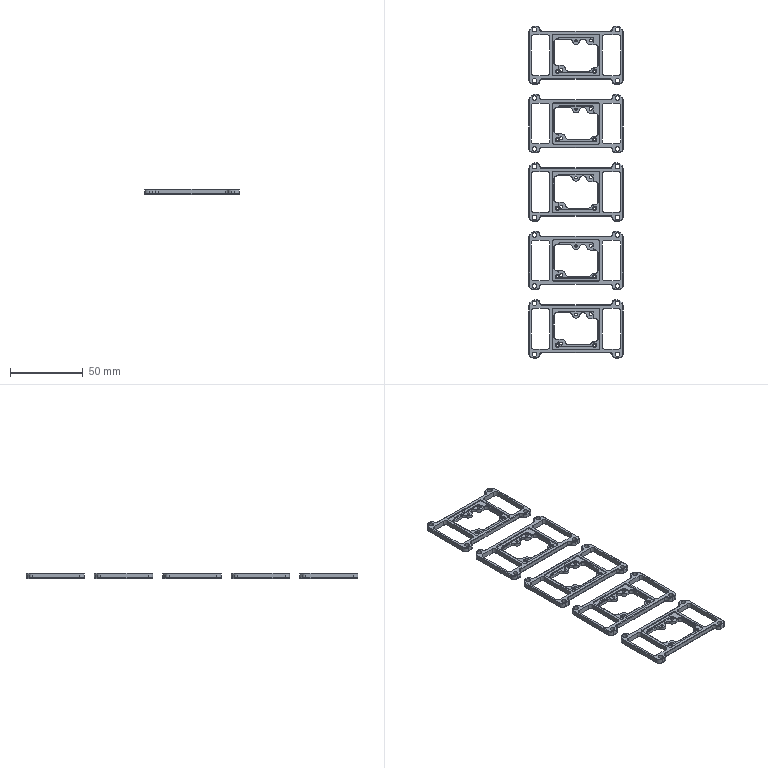Part | 5 solids | 970 faces | box 65 x 228 x 3.5 mm | volume 14203 mm3 | cylinder 395 | plane 335 | cone 170 | torus 70 | commonest cylinder face diameters 4 x125 1 x80 3.2 x40 6 x40 1.6 x30 2 x30